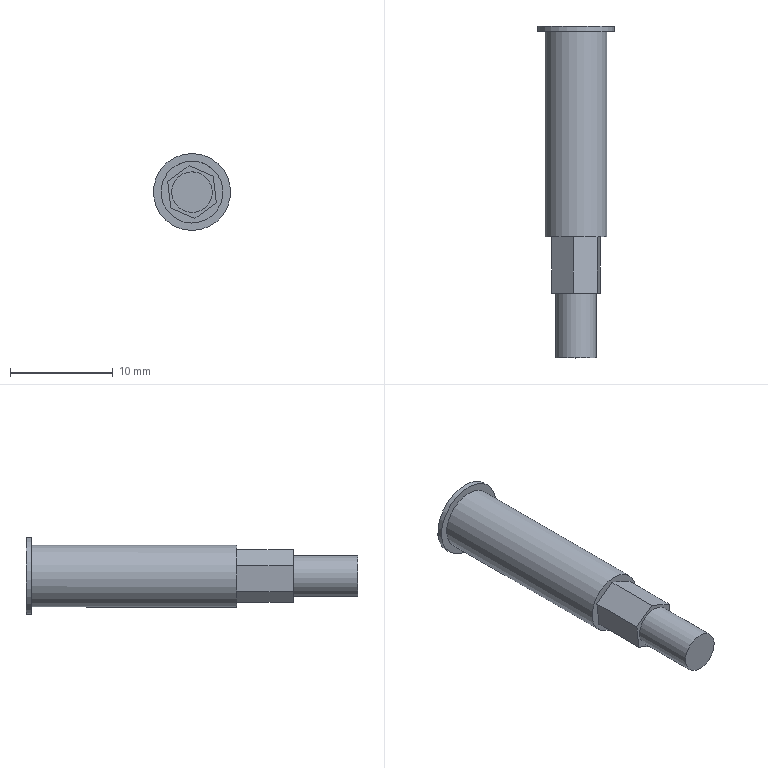Part | STEP file | Dodanie-wyci_gni_cie4_2 | 1 solid | 14 faces | box 7.5 x 32.302 x 7.5 mm | volume 765.405 mm3 | plane 11 | cylinder 3 | commonest cylinder face diameters 3.95 x1 6.03 x1 7.5 x1
STEP:
#1=CARTESIAN_POINT('',(0.,0.,0.));
#2=DIRECTION('',(0.,0.,1.));
#3=DIRECTION('',(1.,0.,0.));
#4=AXIS2_PLACEMENT_3D('',#1,#2,#3);
#5=CARTESIAN_POINT('',(158.273,-25.642,-123.21));
#6=VERTEX_POINT('',#5);
#7=CARTESIAN_POINT('',(158.273,-5.642,-123.202));
#8=VERTEX_POINT('',#7);
#9=CARTESIAN_POINT('',(158.273,-25.642,-123.21));
#10=DIRECTION('',(0.,1.,0.0003815));
#11=VECTOR('',#10,1.);
#12=LINE('',#9,#11);
#13=CARTESIAN_POINT('',(160.724,-5.642,-124.957));
#14=DIRECTION('',(0.,-1.,-0.0003815));
#15=DIRECTION('',(-0.8131,-0.0002221,0.5822));
#16=AXIS2_PLACEMENT_3D('',#13,#14,#15);
#17=CYLINDRICAL_SURFACE('',#16,3.015);
#18=CARTESIAN_POINT('',(0.000000001,20.));
#19=DIRECTION('',(0.,-1.));
#20=VECTOR('',#19,1.);
#21=LINE('',#18,#20);
#22=(GEOMETRIC_REPRESENTATION_CONTEXT(2)PARAMETRIC_REPRESENTATION_CONTEXT()REPRESENTATION_CONTEXT('',''));
#23=DEFINITIONAL_REPRESENTATION('',(#21),#22);
#24=PCURVE('',#17,#23);
#25=CARTESIAN_POINT('',(6.283,20.));
#26=DIRECTION('',(0.,-1.));
#27=VECTOR('',#26,1.);
#28=LINE('',#25,#27);
#29=(GEOMETRIC_REPRESENTATION_CONTEXT(2)PARAMETRIC_REPRESENTATION_CONTEXT()REPRESENTATION_CONTEXT('',''));
#30=DEFINITIONAL_REPRESENTATION('',(#28),#29);
#31=PCURVE('',#17,#30);
#32=SEAM_CURVE('',#12,(#24,#31),.PCURVE_S1.);
#33=EDGE_CURVE('',#6,#8,#32,.T.);
#34=ORIENTED_EDGE('',*,*,#33,.T.);
#35=CARTESIAN_POINT('',(160.724,-5.642,-124.957));
#36=DIRECTION('',(0.,-1.,-0.0003815));
#37=DIRECTION('',(-0.8131,-0.0002221,0.5822));
#38=AXIS2_PLACEMENT_3D('',#35,#36,#37);
#39=CIRCLE('',#38,3.015);
#40=CARTESIAN_POINT('',(0.,0.));
#41=DIRECTION('',(1.,0.));
#42=VECTOR('',#41,1.);
#43=LINE('',#40,#42);
#44=(GEOMETRIC_REPRESENTATION_CONTEXT(2)PARAMETRIC_REPRESENTATION_CONTEXT()REPRESENTATION_CONTEXT('',''));
#45=DEFINITIONAL_REPRESENTATION('',(#43),#44);
#46=PCURVE('',#17,#45);
#47=CARTESIAN_POINT('',(160.724,-5.642,-124.957));
#48=DIRECTION('',(0.,1.,0.0003815));
#49=DIRECTION('',(0.8131,0.0002221,-0.5822));
#50=AXIS2_PLACEMENT_3D('',#47,#48,#49);
#51=PLANE('',#50);
#52=CARTESIAN_POINT('',(-3.015,0.));
#53=CARTESIAN_POINT('',(-3.015,5.222));
#54=CARTESIAN_POINT('',(1.508,2.611));
#55=CARTESIAN_POINT('',(6.03,0.));
#56=CARTESIAN_POINT('',(1.508,-2.611));
#57=CARTESIAN_POINT('',(-3.015,-5.222));
#58=CARTESIAN_POINT('',(-3.015,0.));
#59=(BOUNDED_CURVE()B_SPLINE_CURVE(2,(#52,#53,#54,#55,#56,#57,#58),.UNSPECIFIED.,.T.,.F.)B_SPLINE_CURVE_WITH_KNOTS((1,2,2,2,2,1),(-2.094,0.,2.094,4.189,6.283,8.378),.UNSPECIFIED.)CURVE()GEOMETRIC_REPRESENTATION_ITEM()RATIONAL_B_SPLINE_CURVE((1.,0.5,1.,0.5,1.,0.5,1.))REPRESENTATION_ITEM(''));
#60=(GEOMETRIC_REPRESENTATION_CONTEXT(2)PARAMETRIC_REPRESENTATION_CONTEXT()REPRESENTATION_CONTEXT('',''));
#61=DEFINITIONAL_REPRESENTATION('',(#59),#60);
#62=PCURVE('',#51,#61);
#63=SURFACE_CURVE('',#39,(#46,#62),.PCURVE_S1.);
#64=EDGE_CURVE('',#8,#8,#63,.T.);
#65=ORIENTED_EDGE('',*,*,#64,.T.);
#66=ORIENTED_EDGE('',*,*,#33,.F.);
#67=CARTESIAN_POINT('',(160.724,-25.642,-124.965));
#68=DIRECTION('',(0.,1.,0.0003815));
#69=DIRECTION('',(-0.8131,-0.0002221,0.5822));
#70=AXIS2_PLACEMENT_3D('',#67,#68,#69);
#71=CIRCLE('',#70,3.015);
#72=CARTESIAN_POINT('',(6.283,20.));
#73=DIRECTION('',(-1.,0.));
#74=VECTOR('',#73,1.);
#75=LINE('',#72,#74);
#76=(GEOMETRIC_REPRESENTATION_CONTEXT(2)PARAMETRIC_REPRESENTATION_CONTEXT()REPRESENTATION_CONTEXT('',''));
#77=DEFINITIONAL_REPRESENTATION('',(#75),#76);
#78=PCURVE('',#17,#77);
#79=CARTESIAN_POINT('',(160.724,-25.642,-124.965));
#80=DIRECTION('',(0.,1.,0.0003815));
#81=DIRECTION('',(0.8131,0.0002221,-0.5822));
#82=AXIS2_PLACEMENT_3D('',#79,#80,#81);
#83=PLANE('',#82);
#84=CARTESIAN_POINT('',(0.,0.));
#85=DIRECTION('',(-1.,0.));
#86=AXIS2_PLACEMENT_2D('',#84,#85);
#87=CIRCLE('',#86,3.015);
#88=(GEOMETRIC_REPRESENTATION_CONTEXT(2)PARAMETRIC_REPRESENTATION_CONTEXT()REPRESENTATION_CONTEXT('',''));
#89=DEFINITIONAL_REPRESENTATION('',(#87),#88);
#90=PCURVE('',#83,#89);
#91=SURFACE_CURVE('',#71,(#78,#90),.PCURVE_S1.);
#92=EDGE_CURVE('',#6,#6,#91,.T.);
#93=ORIENTED_EDGE('',*,*,#92,.T.);
#94=EDGE_LOOP('',(#34,#65,#66,#93));
#95=FACE_BOUND('',#94,.T.);
#96=ADVANCED_FACE('',(#95),#17,.T.);
#97=CARTESIAN_POINT('',(157.675,-5.643,-122.774));
#98=VERTEX_POINT('',#97);
#99=CARTESIAN_POINT('',(157.675,-5.143,-122.774));
#100=VERTEX_POINT('',#99);
#101=CARTESIAN_POINT('',(157.675,-5.643,-122.774));
#102=DIRECTION('',(0.,1.,0.0003815));
#103=VECTOR('',#102,1.);
#104=LINE('',#101,#103);
#105=CARTESIAN_POINT('',(160.724,-5.142,-124.957));
#106=DIRECTION('',(0.,-1.,-0.0003815));
#107=DIRECTION('',(-0.8131,-0.0002221,0.5822));
#108=AXIS2_PLACEMENT_3D('',#105,#106,#107);
#109=CYLINDRICAL_SURFACE('',#108,3.75);
#110=CARTESIAN_POINT('',(0.,0.5));
#111=DIRECTION('',(0.,-1.));
#112=VECTOR('',#111,1.);
#113=LINE('',#110,#112);
#114=(GEOMETRIC_REPRESENTATION_CONTEXT(2)PARAMETRIC_REPRESENTATION_CONTEXT()REPRESENTATION_CONTEXT('',''));
#115=DEFINITIONAL_REPRESENTATION('',(#113),#114);
#116=PCURVE('',#109,#115);
#117=CARTESIAN_POINT('',(6.283,0.5));
#118=DIRECTION('',(0.,-1.));
#119=VECTOR('',#118,1.);
#120=LINE('',#117,#119);
#121=(GEOMETRIC_REPRESENTATION_CONTEXT(2)PARAMETRIC_REPRESENTATION_CONTEXT()REPRESENTATION_CONTEXT('',''));
#122=DEFINITIONAL_REPRESENTATION('',(#120),#121);
#123=PCURVE('',#109,#122);
#124=SEAM_CURVE('',#104,(#116,#123),.PCURVE_S1.);
#125=EDGE_CURVE('',#98,#100,#124,.T.);
#126=ORIENTED_EDGE('',*,*,#125,.T.);
#127=CARTESIAN_POINT('',(160.724,-5.142,-124.957));
#128=DIRECTION('',(0.,-1.,-0.0003815));
#129=DIRECTION('',(-0.8131,-0.0002221,0.5822));
#130=AXIS2_PLACEMENT_3D('',#127,#128,#129);
#131=CIRCLE('',#130,3.75);
#132=CARTESIAN_POINT('',(0.,0.));
#133=DIRECTION('',(1.,0.));
#134=VECTOR('',#133,1.);
#135=LINE('',#132,#134);
#136=(GEOMETRIC_REPRESENTATION_CONTEXT(2)PARAMETRIC_REPRESENTATION_CONTEXT()REPRESENTATION_CONTEXT('',''));
#137=DEFINITIONAL_REPRESENTATION('',(#135),#136);
#138=PCURVE('',#109,#137);
#139=CARTESIAN_POINT('',(160.724,-5.142,-124.957));
#140=DIRECTION('',(0.,1.,0.0003815));
#141=DIRECTION('',(0.8131,0.0002221,-0.5822));
#142=AXIS2_PLACEMENT_3D('',#139,#140,#141);
#143=PLANE('',#142);
#144=CARTESIAN_POINT('',(-3.75,0.));
#145=CARTESIAN_POINT('',(-3.75,6.495));
#146=CARTESIAN_POINT('',(1.875,3.248));
#147=CARTESIAN_POINT('',(7.5,0.));
#148=CARTESIAN_POINT('',(1.875,-3.248));
#149=CARTESIAN_POINT('',(-3.75,-6.495));
#150=CARTESIAN_POINT('',(-3.75,0.));
#151=(BOUNDED_CURVE()B_SPLINE_CURVE(2,(#144,#145,#146,#147,#148,#149,#150),.UNSPECIFIED.,.T.,.F.)B_SPLINE_CURVE_WITH_KNOTS((1,2,2,2,2,1),(-2.094,0.,2.094,4.189,6.283,8.378),.UNSPECIFIED.)CURVE()GEOMETRIC_REPRESENTATION_ITEM()RATIONAL_B_SPLINE_CURVE((1.,0.5,1.,0.5,1.,0.5,1.))REPRESENTATION_ITEM(''));
#152=(GEOMETRIC_REPRESENTATION_CONTEXT(2)PARAMETRIC_REPRESENTATION_CONTEXT()REPRESENTATION_CONTEXT('',''));
#153=DEFINITIONAL_REPRESENTATION('',(#151),#152);
#154=PCURVE('',#143,#153);
#155=SURFACE_CURVE('',#131,(#138,#154),.PCURVE_S1.);
#156=EDGE_CURVE('',#100,#100,#155,.T.);
#157=ORIENTED_EDGE('',*,*,#156,.T.);
#158=ORIENTED_EDGE('',*,*,#125,.F.);
#159=CARTESIAN_POINT('',(160.724,-5.642,-124.957));
#160=DIRECTION('',(0.,1.,0.0003815));
#161=DIRECTION('',(-0.8131,-0.0002221,0.5822));
#162=AXIS2_PLACEMENT_3D('',#159,#160,#161);
#163=CIRCLE('',#162,3.75);
#164=CARTESIAN_POINT('',(6.283,0.5));
#165=DIRECTION('',(-1.,0.));
#166=VECTOR('',#165,1.);
#167=LINE('',#164,#166);
#168=(GEOMETRIC_REPRESENTATION_CONTEXT(2)PARAMETRIC_REPRESENTATION_CONTEXT()REPRESENTATION_CONTEXT('',''));
#169=DEFINITIONAL_REPRESENTATION('',(#167),#168);
#170=PCURVE('',#109,#169);
#171=CARTESIAN_POINT('',(0.,0.));
#172=DIRECTION('',(-1.,0.));
#173=AXIS2_PLACEMENT_2D('',#171,#172);
#174=CIRCLE('',#173,3.75);
#175=(GEOMETRIC_REPRESENTATION_CONTEXT(2)PARAMETRIC_REPRESENTATION_CONTEXT()REPRESENTATION_CONTEXT('',''));
#176=DEFINITIONAL_REPRESENTATION('',(#174),#175);
#177=PCURVE('',#51,#176);
#178=SURFACE_CURVE('',#163,(#170,#177),.PCURVE_S1.);
#179=EDGE_CURVE('',#98,#98,#178,.T.);
#180=ORIENTED_EDGE('',*,*,#179,.T.);
#181=EDGE_LOOP('',(#126,#157,#158,#180));
#182=FACE_BOUND('',#181,.T.);
#183=ADVANCED_FACE('',(#182),#109,.T.);
#184=CARTESIAN_POINT('',(159.118,-37.442,-123.82));
#185=VERTEX_POINT('',#184);
#186=CARTESIAN_POINT('',(159.118,-31.142,-123.817));
#187=VERTEX_POINT('',#186);
#188=CARTESIAN_POINT('',(159.118,-37.442,-123.82));
#189=DIRECTION('',(0.,1.,0.0003815));
#190=VECTOR('',#189,1.);
#191=LINE('',#188,#190);
#192=CARTESIAN_POINT('',(160.724,-31.142,-124.967));
#193=DIRECTION('',(0.,-1.,-0.0003815));
#194=DIRECTION('',(-0.8131,-0.0002221,0.5822));
#195=AXIS2_PLACEMENT_3D('',#192,#193,#194);
#196=CYLINDRICAL_SURFACE('',#195,1.975);
#197=CARTESIAN_POINT('',(0.,6.3));
#198=DIRECTION('',(0.,-1.));
#199=VECTOR('',#198,1.);
#200=LINE('',#197,#199);
#201=(GEOMETRIC_REPRESENTATION_CONTEXT(2)PARAMETRIC_REPRESENTATION_CONTEXT()REPRESENTATION_CONTEXT('',''));
#202=DEFINITIONAL_REPRESENTATION('',(#200),#201);
#203=PCURVE('',#196,#202);
#204=CARTESIAN_POINT('',(6.283,6.3));
#205=DIRECTION('',(0.,-1.));
#206=VECTOR('',#205,1.);
#207=LINE('',#204,#206);
#208=(GEOMETRIC_REPRESENTATION_CONTEXT(2)PARAMETRIC_REPRESENTATION_CONTEXT()REPRESENTATION_CONTEXT('',''));
#209=DEFINITIONAL_REPRESENTATION('',(#207),#208);
#210=PCURVE('',#196,#209);
#211=SEAM_CURVE('',#191,(#203,#210),.PCURVE_S1.);
#212=EDGE_CURVE('',#185,#187,#211,.T.);
#213=ORIENTED_EDGE('',*,*,#212,.T.);
#214=CARTESIAN_POINT('',(160.724,-31.142,-124.967));
#215=DIRECTION('',(0.,-1.,-0.0003815));
#216=DIRECTION('',(-0.8131,-0.0002221,0.5822));
#217=AXIS2_PLACEMENT_3D('',#214,#215,#216);
#218=CIRCLE('',#217,1.975);
#219=CARTESIAN_POINT('',(0.,0.));
#220=DIRECTION('',(1.,0.));
#221=VECTOR('',#220,1.);
#222=LINE('',#219,#221);
#223=(GEOMETRIC_REPRESENTATION_CONTEXT(2)PARAMETRIC_REPRESENTATION_CONTEXT()REPRESENTATION_CONTEXT('',''));
#224=DEFINITIONAL_REPRESENTATION('',(#222),#223);
#225=PCURVE('',#196,#224);
#226=CARTESIAN_POINT('',(160.724,-31.142,-124.967));
#227=DIRECTION('',(0.,1.,0.0003815));
#228=DIRECTION('',(0.8131,0.0002221,-0.5822));
#229=AXIS2_PLACEMENT_3D('',#226,#227,#228);
#230=PLANE('',#229);
#231=CARTESIAN_POINT('',(-1.975,0.));
#232=CARTESIAN_POINT('',(-1.975,3.421));
#233=CARTESIAN_POINT('',(0.9875,1.71));
#234=CARTESIAN_POINT('',(3.95,0.));
#235=CARTESIAN_POINT('',(0.9875,-1.71));
#236=CARTESIAN_POINT('',(-1.975,-3.421));
#237=CARTESIAN_POINT('',(-1.975,0.));
#238=(BOUNDED_CURVE()B_SPLINE_CURVE(2,(#231,#232,#233,#234,#235,#236,#237),.UNSPECIFIED.,.T.,.F.)B_SPLINE_CURVE_WITH_KNOTS((1,2,2,2,2,1),(-2.094,0.,2.094,4.189,6.283,8.378),.UNSPECIFIED.)CURVE()GEOMETRIC_REPRESENTATION_ITEM()RATIONAL_B_SPLINE_CURVE((1.,0.5,1.,0.5,1.,0.5,1.))REPRESENTATION_ITEM(''));
#239=(GEOMETRIC_REPRESENTATION_CONTEXT(2)PARAMETRIC_REPRESENTATION_CONTEXT()REPRESENTATION_CONTEXT('',''));
#240=DEFINITIONAL_REPRESENTATION('',(#238),#239);
#241=PCURVE('',#230,#240);
#242=SURFACE_CURVE('',#218,(#225,#241),.PCURVE_S1.);
#243=EDGE_CURVE('',#187,#187,#242,.T.);
#244=ORIENTED_EDGE('',*,*,#243,.T.);
#245=ORIENTED_EDGE('',*,*,#212,.F.);
#246=CARTESIAN_POINT('',(160.724,-37.442,-124.969));
#247=DIRECTION('',(0.,1.,0.0003815));
#248=DIRECTION('',(-0.8131,-0.0002221,0.5822));
#249=AXIS2_PLACEMENT_3D('',#246,#247,#248);
#250=CIRCLE('',#249,1.975);
#251=CARTESIAN_POINT('',(6.283,6.3));
#252=DIRECTION('',(-1.,0.));
#253=VECTOR('',#252,1.);
#254=LINE('',#251,#253);
#255=(GEOMETRIC_REPRESENTATION_CONTEXT(2)PARAMETRIC_REPRESENTATION_CONTEXT()REPRESENTATION_CONTEXT('',''));
#256=DEFINITIONAL_REPRESENTATION('',(#254),#255);
#257=PCURVE('',#196,#256);
#258=CARTESIAN_POINT('',(160.724,-37.442,-124.969));
#259=DIRECTION('',(0.,1.,0.0003815));
#260=DIRECTION('',(0.8131,0.0002221,-0.5822));
#261=AXIS2_PLACEMENT_3D('',#258,#259,#260);
#262=PLANE('',#261);
#263=CARTESIAN_POINT('',(0.,0.));
#264=DIRECTION('',(-1.,0.));
#265=AXIS2_PLACEMENT_2D('',#263,#264);
#266=CIRCLE('',#265,1.975);
#267=(GEOMETRIC_REPRESENTATION_CONTEXT(2)PARAMETRIC_REPRESENTATION_CONTEXT()REPRESENTATION_CONTEXT('',''));
#268=DEFINITIONAL_REPRESENTATION('',(#266),#267);
#269=PCURVE('',#262,#268);
#270=SURFACE_CURVE('',#250,(#257,#269),.PCURVE_S1.);
#271=EDGE_CURVE('',#185,#185,#270,.T.);
#272=ORIENTED_EDGE('',*,*,#271,.T.);
#273=EDGE_LOOP('',(#213,#244,#245,#272));
#274=FACE_BOUND('',#273,.T.);
#275=ADVANCED_FACE('',(#274),#196,.T.);
#276=CARTESIAN_POINT('',(161.015,-25.641,-127.526));
#277=VERTEX_POINT('',#276);
#278=CARTESIAN_POINT('',(163.088,-25.641,-125.994));
#279=VERTEX_POINT('',#278);
#280=CARTESIAN_POINT('',(161.015,-25.641,-127.526));
#281=DIRECTION('',(0.8042,-0.0002268,0.5944));
#282=VECTOR('',#281,1.);
#283=LINE('',#280,#282);
#284=CARTESIAN_POINT('',(1.727,1.913));
#285=DIRECTION('',(0.3078,-0.9515));
#286=VECTOR('',#285,1.);
#287=LINE('',#284,#286);
#288=(GEOMETRIC_REPRESENTATION_CONTEXT(2)PARAMETRIC_REPRESENTATION_CONTEXT()REPRESENTATION_CONTEXT('',''));
#289=DEFINITIONAL_REPRESENTATION('',(#287),#288);
#290=PCURVE('',#83,#289);
#291=CARTESIAN_POINT('',(162.051,-28.391,-126.761));
#292=DIRECTION('',(-0.5944,-0.0003068,0.8042));
#293=DIRECTION('',(0.8042,-0.0002268,0.5944));
#294=AXIS2_PLACEMENT_3D('',#291,#292,#293);
#295=PLANE('',#294);
#296=CARTESIAN_POINT('',(-1.289,2.75));
#297=DIRECTION('',(1.,0.));
#298=VECTOR('',#297,1.);
#299=LINE('',#296,#298);
#300=(GEOMETRIC_REPRESENTATION_CONTEXT(2)PARAMETRIC_REPRESENTATION_CONTEXT()REPRESENTATION_CONTEXT('',''));
#301=DEFINITIONAL_REPRESENTATION('',(#299),#300);
#302=PCURVE('',#295,#301);
#303=SURFACE_CURVE('',#283,(#290,#302),.PCURVE_S1.);
#304=EDGE_CURVE('',#277,#279,#303,.T.);
#305=ORIENTED_EDGE('',*,*,#304,.F.);
#306=CARTESIAN_POINT('',(158.651,-25.641,-126.497));
#307=VERTEX_POINT('',#306);
#308=CARTESIAN_POINT('',(158.651,-25.641,-126.497));
#309=DIRECTION('',(0.9169,0.0001523,-0.3992));
#310=VECTOR('',#309,1.);
#311=LINE('',#308,#310);
#312=CARTESIAN_POINT('',(-0.7934,2.453));
#313=DIRECTION('',(0.9779,-0.2092));
#314=VECTOR('',#313,1.);
#315=LINE('',#312,#314);
#316=(GEOMETRIC_REPRESENTATION_CONTEXT(2)PARAMETRIC_REPRESENTATION_CONTEXT()REPRESENTATION_CONTEXT('',''));
#317=DEFINITIONAL_REPRESENTATION('',(#315),#316);
#318=PCURVE('',#83,#317);
#319=CARTESIAN_POINT('',(159.833,-28.391,-127.013));
#320=DIRECTION('',(0.3992,-0.0003498,0.9169));
#321=DIRECTION('',(0.9169,0.0001523,-0.3992));
#322=AXIS2_PLACEMENT_3D('',#319,#320,#321);
#323=PLANE('',#322);
#324=CARTESIAN_POINT('',(-1.289,2.75));
#325=DIRECTION('',(1.,0.));
#326=VECTOR('',#325,1.);
#327=LINE('',#324,#326);
#328=(GEOMETRIC_REPRESENTATION_CONTEXT(2)PARAMETRIC_REPRESENTATION_CONTEXT()REPRESENTATION_CONTEXT('',''));
#329=DEFINITIONAL_REPRESENTATION('',(#327),#328);
#330=PCURVE('',#323,#329);
#331=SURFACE_CURVE('',#311,(#318,#330),.PCURVE_S1.);
#332=EDGE_CURVE('',#307,#277,#331,.T.);
#333=ORIENTED_EDGE('',*,*,#332,.F.);
#334=CARTESIAN_POINT('',(158.361,-25.642,-123.936));
#335=VERTEX_POINT('',#334);
#336=CARTESIAN_POINT('',(158.361,-25.642,-123.936));
#337=DIRECTION('',(0.1127,0.000379,-0.9936));
#338=VECTOR('',#337,1.);
#339=LINE('',#336,#338);
#340=CARTESIAN_POINT('',(-2.521,0.5392));
#341=DIRECTION('',(0.6701,0.7423));
#342=VECTOR('',#341,1.);
#343=LINE('',#340,#342);
#344=(GEOMETRIC_REPRESENTATION_CONTEXT(2)PARAMETRIC_REPRESENTATION_CONTEXT()REPRESENTATION_CONTEXT('',''));
#345=DEFINITIONAL_REPRESENTATION('',(#343),#344);
#346=PCURVE('',#83,#345);
#347=CARTESIAN_POINT('',(158.506,-28.392,-125.218));
#348=DIRECTION('',(0.9936,-0.00004299,0.1127));
#349=DIRECTION('',(0.1127,0.000379,-0.9936));
#350=AXIS2_PLACEMENT_3D('',#347,#348,#349);
#351=PLANE('',#350);
#352=CARTESIAN_POINT('',(-1.289,2.75));
#353=DIRECTION('',(1.,0.));
#354=VECTOR('',#353,1.);
#355=LINE('',#352,#354);
#356=(GEOMETRIC_REPRESENTATION_CONTEXT(2)PARAMETRIC_REPRESENTATION_CONTEXT()REPRESENTATION_CONTEXT('',''));
#357=DEFINITIONAL_REPRESENTATION('',(#355),#356);
#358=PCURVE('',#351,#357);
#359=SURFACE_CURVE('',#339,(#346,#358),.PCURVE_S1.);
#360=EDGE_CURVE('',#335,#307,#359,.T.);
#361=ORIENTED_EDGE('',*,*,#360,.F.);
#362=CARTESIAN_POINT('',(160.434,-25.643,-122.404));
#363=VERTEX_POINT('',#362);
#364=CARTESIAN_POINT('',(160.434,-25.643,-122.404));
#365=DIRECTION('',(-0.8042,0.0002268,-0.5944));
#366=VECTOR('',#365,1.);
#367=LINE('',#364,#366);
#368=CARTESIAN_POINT('',(-1.727,-1.913));
#369=DIRECTION('',(-0.3078,0.9515));
#370=VECTOR('',#369,1.);
#371=LINE('',#368,#370);
#372=(GEOMETRIC_REPRESENTATION_CONTEXT(2)PARAMETRIC_REPRESENTATION_CONTEXT()REPRESENTATION_CONTEXT('',''));
#373=DEFINITIONAL_REPRESENTATION('',(#371),#372);
#374=PCURVE('',#83,#373);
#375=CARTESIAN_POINT('',(159.397,-28.392,-123.171));
#376=DIRECTION('',(0.5944,0.0003068,-0.8042));
#377=DIRECTION('',(-0.8042,0.0002268,-0.5944));
#378=AXIS2_PLACEMENT_3D('',#375,#376,#377);
#379=PLANE('',#378);
#380=CARTESIAN_POINT('',(-1.289,2.75));
#381=DIRECTION('',(1.,0.));
#382=VECTOR('',#381,1.);
#383=LINE('',#380,#382);
#384=(GEOMETRIC_REPRESENTATION_CONTEXT(2)PARAMETRIC_REPRESENTATION_CONTEXT()REPRESENTATION_CONTEXT('',''));
#385=DEFINITIONAL_REPRESENTATION('',(#383),#384);
#386=PCURVE('',#379,#385);
#387=SURFACE_CURVE('',#367,(#374,#386),.PCURVE_S1.);
#388=EDGE_CURVE('',#363,#335,#387,.T.);
#389=ORIENTED_EDGE('',*,*,#388,.F.);
#390=CARTESIAN_POINT('',(162.797,-25.642,-123.433));
#391=VERTEX_POINT('',#390);
#392=CARTESIAN_POINT('',(162.797,-25.642,-123.433));
#393=DIRECTION('',(-0.9169,-0.0001523,0.3992));
#394=VECTOR('',#393,1.);
#395=LINE('',#392,#394);
#396=CARTESIAN_POINT('',(0.7934,-2.453));
#397=DIRECTION('',(-0.9779,0.2092));
#398=VECTOR('',#397,1.);
#399=LINE('',#396,#398);
#400=(GEOMETRIC_REPRESENTATION_CONTEXT(2)PARAMETRIC_REPRESENTATION_CONTEXT()REPRESENTATION_CONTEXT('',''));
#401=DEFINITIONAL_REPRESENTATION('',(#399),#400);
#402=PCURVE('',#83,#401);
#403=CARTESIAN_POINT('',(161.615,-28.393,-122.919));
#404=DIRECTION('',(-0.3992,0.0003498,-0.9169));
#405=DIRECTION('',(-0.9169,-0.0001523,0.3992));
#406=AXIS2_PLACEMENT_3D('',#403,#404,#405);
#407=PLANE('',#406);
#408=CARTESIAN_POINT('',(-1.289,2.75));
#409=DIRECTION('',(1.,0.));
#410=VECTOR('',#409,1.);
#411=LINE('',#408,#410);
#412=(GEOMETRIC_REPRESENTATION_CONTEXT(2)PARAMETRIC_REPRESENTATION_CONTEXT()REPRESENTATION_CONTEXT('',''));
#413=DEFINITIONAL_REPRESENTATION('',(#411),#412);
#414=PCURVE('',#407,#413);
#415=SURFACE_CURVE('',#395,(#402,#414),.PCURVE_S1.);
#416=EDGE_CURVE('',#391,#363,#415,.T.);
#417=ORIENTED_EDGE('',*,*,#416,.F.);
#418=CARTESIAN_POINT('',(163.088,-25.641,-125.994));
#419=DIRECTION('',(-0.1127,-0.000379,0.9936));
#420=VECTOR('',#419,1.);
#421=LINE('',#418,#420);
#422=CARTESIAN_POINT('',(2.521,-0.5392));
#423=DIRECTION('',(-0.6701,-0.7423));
#424=VECTOR('',#423,1.);
#425=LINE('',#422,#424);
#426=(GEOMETRIC_REPRESENTATION_CONTEXT(2)PARAMETRIC_REPRESENTATION_CONTEXT()REPRESENTATION_CONTEXT('',''));
#427=DEFINITIONAL_REPRESENTATION('',(#425),#426);
#428=PCURVE('',#83,#427);
#429=CARTESIAN_POINT('',(162.942,-28.392,-124.714));
#430=DIRECTION('',(-0.9936,0.00004299,-0.1127));
#431=DIRECTION('',(-0.1127,-0.000379,0.9936));
#432=AXIS2_PLACEMENT_3D('',#429,#430,#431);
#433=PLANE('',#432);
#434=CARTESIAN_POINT('',(-1.289,2.75));
#435=DIRECTION('',(1.,0.));
#436=VECTOR('',#435,1.);
#437=LINE('',#434,#436);
#438=(GEOMETRIC_REPRESENTATION_CONTEXT(2)PARAMETRIC_REPRESENTATION_CONTEXT()REPRESENTATION_CONTEXT('',''));
#439=DEFINITIONAL_REPRESENTATION('',(#437),#438);
#440=PCURVE('',#433,#439);
#441=SURFACE_CURVE('',#421,(#428,#440),.PCURVE_S1.);
#442=EDGE_CURVE('',#279,#391,#441,.T.);
#443=ORIENTED_EDGE('',*,*,#442,.F.);
#444=EDGE_LOOP('',(#305,#333,#361,#389,#417,#443));
#445=FACE_BOUND('',#444,.T.);
#446=ORIENTED_EDGE('',*,*,#92,.F.);
#447=EDGE_LOOP('',(#446));
#448=FACE_BOUND('',#447,.T.);
#449=ADVANCED_FACE('',(#445,#448),#83,.F.);
#450=ORIENTED_EDGE('',*,*,#64,.F.);
#451=EDGE_LOOP('',(#450));
#452=FACE_BOUND('',#451,.T.);
#453=ORIENTED_EDGE('',*,*,#179,.F.);
#454=EDGE_LOOP('',(#453));
#455=FACE_BOUND('',#454,.T.);
#456=ADVANCED_FACE('',(#452,#455),#51,.F.);
#457=CARTESIAN_POINT('',(163.088,-31.141,-125.996));
#458=VERTEX_POINT('',#457);
#459=CARTESIAN_POINT('',(163.088,-25.641,-125.994));
#460=DIRECTION('',(0.,-1.,-0.0003815));
#461=VECTOR('',#460,1.);
#462=LINE('',#459,#461);
#463=CARTESIAN_POINT('',(-1.289,2.75));
#464=DIRECTION('',(0.,-1.));
#465=VECTOR('',#464,1.);
#466=LINE('',#463,#465);
#467=(GEOMETRIC_REPRESENTATION_CONTEXT(2)PARAMETRIC_REPRESENTATION_CONTEXT()REPRESENTATION_CONTEXT('',''));
#468=DEFINITIONAL_REPRESENTATION('',(#466),#467);
#469=PCURVE('',#433,#468);
#470=CARTESIAN_POINT('',(1.289,2.75));
#471=DIRECTION('',(0.,-1.));
#472=VECTOR('',#471,1.);
#473=LINE('',#470,#472);
#474=(GEOMETRIC_REPRESENTATION_CONTEXT(2)PARAMETRIC_REPRESENTATION_CONTEXT()REPRESENTATION_CONTEXT('',''));
#475=DEFINITIONAL_REPRESENTATION('',(#473),#474);
#476=PCURVE('',#295,#475);
#477=SURFACE_CURVE('',#462,(#469,#476),.PCURVE_S1.);
#478=EDGE_CURVE('',#279,#458,#477,.T.);
#479=ORIENTED_EDGE('',*,*,#478,.F.);
#480=ORIENTED_EDGE('',*,*,#442,.T.);
#481=CARTESIAN_POINT('',(162.797,-31.142,-123.435));
#482=VERTEX_POINT('',#481);
#483=CARTESIAN_POINT('',(162.797,-31.142,-123.435));
#484=DIRECTION('',(0.,1.,0.0003815));
#485=VECTOR('',#484,1.);
#486=LINE('',#483,#485);
#487=CARTESIAN_POINT('',(1.289,-2.75));
#488=DIRECTION('',(0.,1.));
#489=VECTOR('',#488,1.);
#490=LINE('',#487,#489);
#491=(GEOMETRIC_REPRESENTATION_CONTEXT(2)PARAMETRIC_REPRESENTATION_CONTEXT()REPRESENTATION_CONTEXT('',''));
#492=DEFINITIONAL_REPRESENTATION('',(#490),#491);
#493=PCURVE('',#433,#492);
#494=CARTESIAN_POINT('',(-1.289,-2.75));
#495=DIRECTION('',(0.,1.));
#496=VECTOR('',#495,1.);
#497=LINE('',#494,#496);
#498=(GEOMETRIC_REPRESENTATION_CONTEXT(2)PARAMETRIC_REPRESENTATION_CONTEXT()REPRESENTATION_CONTEXT('',''));
#499=DEFINITIONAL_REPRESENTATION('',(#497),#498);
#500=PCURVE('',#407,#499);
#501=SURFACE_CURVE('',#486,(#493,#500),.PCURVE_S1.);
#502=EDGE_CURVE('',#482,#391,#501,.T.);
#503=ORIENTED_EDGE('',*,*,#502,.F.);
#504=CARTESIAN_POINT('',(163.088,-31.141,-125.996));
#505=DIRECTION('',(-0.1127,-0.000379,0.9936));
#506=VECTOR('',#505,1.);
#507=LINE('',#504,#506);
#508=CARTESIAN_POINT('',(-1.289,-2.75));
#509=DIRECTION('',(1.,0.));
#510=VECTOR('',#509,1.);
#511=LINE('',#508,#510);
#512=(GEOMETRIC_REPRESENTATION_CONTEXT(2)PARAMETRIC_REPRESENTATION_CONTEXT()REPRESENTATION_CONTEXT('',''));
#513=DEFINITIONAL_REPRESENTATION('',(#511),#512);
#514=PCURVE('',#433,#513);
#515=CARTESIAN_POINT('',(2.521,-0.5392));
#516=DIRECTION('',(-0.6701,-0.7423));
#517=VECTOR('',#516,1.);
#518=LINE('',#515,#517);
#519=(GEOMETRIC_REPRESENTATION_CONTEXT(2)PARAMETRIC_REPRESENTATION_CONTEXT()REPRESENTATION_CONTEXT('',''));
#520=DEFINITIONAL_REPRESENTATION('',(#518),#519);
#521=PCURVE('',#230,#520);
#522=SURFACE_CURVE('',#507,(#514,#521),.PCURVE_S1.);
#523=EDGE_CURVE('',#458,#482,#522,.T.);
#524=ORIENTED_EDGE('',*,*,#523,.F.);
#525=EDGE_LOOP('',(#479,#480,#503,#524));
#526=FACE_BOUND('',#525,.T.);
#527=ADVANCED_FACE('',(#526),#433,.F.);
#528=CARTESIAN_POINT('',(161.015,-31.141,-127.529));
#529=VERTEX_POINT('',#528);
#530=CARTESIAN_POINT('',(161.015,-25.641,-127.526));
#531=DIRECTION('',(0.,-1.,-0.0003815));
#532=VECTOR('',#531,1.);
#533=LINE('',#530,#532);
#534=CARTESIAN_POINT('',(-1.289,2.75));
#535=DIRECTION('',(0.,-1.));
#536=VECTOR('',#535,1.);
#537=LINE('',#534,#536);
#538=(GEOMETRIC_REPRESENTATION_CONTEXT(2)PARAMETRIC_REPRESENTATION_CONTEXT()REPRESENTATION_CONTEXT('',''));
#539=DEFINITIONAL_REPRESENTATION('',(#537),#538);
#540=PCURVE('',#295,#539);
#541=CARTESIAN_POINT('',(1.289,2.75));
#542=DIRECTION('',(0.,-1.));
#543=VECTOR('',#542,1.);
#544=LINE('',#541,#543);
#545=(GEOMETRIC_REPRESENTATION_CONTEXT(2)PARAMETRIC_REPRESENTATION_CONTEXT()REPRESENTATION_CONTEXT('',''));
#546=DEFINITIONAL_REPRESENTATION('',(#544),#545);
#547=PCURVE('',#323,#546);
#548=SURFACE_CURVE('',#533,(#540,#547),.PCURVE_S1.);
#549=EDGE_CURVE('',#277,#529,#548,.T.);
#550=ORIENTED_EDGE('',*,*,#549,.F.);
#551=ORIENTED_EDGE('',*,*,#304,.T.);
#552=ORIENTED_EDGE('',*,*,#478,.T.);
#553=CARTESIAN_POINT('',(161.015,-31.141,-127.529));
#554=DIRECTION('',(0.8042,-0.0002268,0.5944));
#555=VECTOR('',#554,1.);
#556=LINE('',#553,#555);
#557=CARTESIAN_POINT('',(-1.289,-2.75));
#558=DIRECTION('',(1.,0.));
#559=VECTOR('',#558,1.);
#560=LINE('',#557,#559);
#561=(GEOMETRIC_REPRESENTATION_CONTEXT(2)PARAMETRIC_REPRESENTATION_CONTEXT()REPRESENTATION_CONTEXT('',''));
#562=DEFINITIONAL_REPRESENTATION('',(#560),#561);
#563=PCURVE('',#295,#562);
#564=CARTESIAN_POINT('',(1.727,1.913));
#565=DIRECTION('',(0.3078,-0.9515));
#566=VECTOR('',#565,1.);
#567=LINE('',#564,#566);
#568=(GEOMETRIC_REPRESENTATION_CONTEXT(2)PARAMETRIC_REPRESENTATION_CONTEXT()REPRESENTATION_CONTEXT('',''));
#569=DEFINITIONAL_REPRESENTATION('',(#567),#568);
#570=PCURVE('',#230,#569);
#571=SURFACE_CURVE('',#556,(#563,#570),.PCURVE_S1.);
#572=EDGE_CURVE('',#529,#458,#571,.T.);
#573=ORIENTED_EDGE('',*,*,#572,.F.);
#574=EDGE_LOOP('',(#550,#551,#552,#573));
#575=FACE_BOUND('',#574,.T.);
#576=ADVANCED_FACE('',(#575),#295,.F.);
#577=CARTESIAN_POINT('',(158.651,-31.141,-126.499));
#578=VERTEX_POINT('',#577);
#579=CARTESIAN_POINT('',(158.651,-25.641,-126.497));
#580=DIRECTION('',(0.,-1.,-0.0003815));
#581=VECTOR('',#580,1.);
#582=LINE('',#579,#581);
#583=CARTESIAN_POINT('',(-1.289,2.75));
#584=DIRECTION('',(0.,-1.));
#585=VECTOR('',#584,1.);
#586=LINE('',#583,#585);
#587=(GEOMETRIC_REPRESENTATION_CONTEXT(2)PARAMETRIC_REPRESENTATION_CONTEXT()REPRESENTATION_CONTEXT('',''));
#588=DEFINITIONAL_REPRESENTATION('',(#586),#587);
#589=PCURVE('',#323,#588);
#590=CARTESIAN_POINT('',(1.289,2.75));
#591=DIRECTION('',(0.,-1.));
#592=VECTOR('',#591,1.);
#593=LINE('',#590,#592);
#594=(GEOMETRIC_REPRESENTATION_CONTEXT(2)PARAMETRIC_REPRESENTATION_CONTEXT()REPRESENTATION_CONTEXT('',''));
#595=DEFINITIONAL_REPRESENTATION('',(#593),#594);
#596=PCURVE('',#351,#595);
#597=SURFACE_CURVE('',#582,(#589,#596),.PCURVE_S1.);
#598=EDGE_CURVE('',#307,#578,#597,.T.);
#599=ORIENTED_EDGE('',*,*,#598,.F.);
#600=ORIENTED_EDGE('',*,*,#332,.T.);
#601=ORIENTED_EDGE('',*,*,#549,.T.);
#602=CARTESIAN_POINT('',(158.651,-31.141,-126.499));
#603=DIRECTION('',(0.9169,0.0001523,-0.3992));
#604=VECTOR('',#603,1.);
#605=LINE('',#602,#604);
#606=CARTESIAN_POINT('',(-1.289,-2.75));
#607=DIRECTION('',(1.,0.));
#608=VECTOR('',#607,1.);
#609=LINE('',#606,#608);
#610=(GEOMETRIC_REPRESENTATION_CONTEXT(2)PARAMETRIC_REPRESENTATION_CONTEXT()REPRESENTATION_CONTEXT('',''));
#611=DEFINITIONAL_REPRESENTATION('',(#609),#610);
#612=PCURVE('',#323,#611);
#613=CARTESIAN_POINT('',(-0.7934,2.453));
#614=DIRECTION('',(0.9779,-0.2092));
#615=VECTOR('',#614,1.);
#616=LINE('',#613,#615);
#617=(GEOMETRIC_REPRESENTATION_CONTEXT(2)PARAMETRIC_REPRESENTATION_CONTEXT()REPRESENTATION_CONTEXT('',''));
#618=DEFINITIONAL_REPRESENTATION('',(#616),#617);
#619=PCURVE('',#230,#618);
#620=SURFACE_CURVE('',#605,(#612,#619),.PCURVE_S1.);
#621=EDGE_CURVE('',#578,#529,#620,.T.);
#622=ORIENTED_EDGE('',*,*,#621,.F.);
#623=EDGE_LOOP('',(#599,#600,#601,#622));
#624=FACE_BOUND('',#623,.T.);
#625=ADVANCED_FACE('',(#624),#323,.F.);
#626=CARTESIAN_POINT('',(158.361,-31.142,-123.938));
#627=VERTEX_POINT('',#626);
#628=CARTESIAN_POINT('',(158.361,-25.642,-123.936));
#629=DIRECTION('',(0.,-1.,-0.0003815));
#630=VECTOR('',#629,1.);
#631=LINE('',#628,#630);
#632=CARTESIAN_POINT('',(-1.289,2.75));
#633=DIRECTION('',(0.,-1.));
#634=VECTOR('',#633,1.);
#635=LINE('',#632,#634);
#636=(GEOMETRIC_REPRESENTATION_CONTEXT(2)PARAMETRIC_REPRESENTATION_CONTEXT()REPRESENTATION_CONTEXT('',''));
#637=DEFINITIONAL_REPRESENTATION('',(#635),#636);
#638=PCURVE('',#351,#637);
#639=CARTESIAN_POINT('',(1.289,2.75));
#640=DIRECTION('',(0.,-1.));
#641=VECTOR('',#640,1.);
#642=LINE('',#639,#641);
#643=(GEOMETRIC_REPRESENTATION_CONTEXT(2)PARAMETRIC_REPRESENTATION_CONTEXT()REPRESENTATION_CONTEXT('',''));
#644=DEFINITIONAL_REPRESENTATION('',(#642),#643);
#645=PCURVE('',#379,#644);
#646=SURFACE_CURVE('',#631,(#638,#645),.PCURVE_S1.);
#647=EDGE_CURVE('',#335,#627,#646,.T.);
#648=ORIENTED_EDGE('',*,*,#647,.F.);
#649=ORIENTED_EDGE('',*,*,#360,.T.);
#650=ORIENTED_EDGE('',*,*,#598,.T.);
#651=CARTESIAN_POINT('',(158.361,-31.142,-123.938));
#652=DIRECTION('',(0.1127,0.000379,-0.9936));
#653=VECTOR('',#652,1.);
#654=LINE('',#651,#653);
#655=CARTESIAN_POINT('',(-1.289,-2.75));
#656=DIRECTION('',(1.,0.));
#657=VECTOR('',#656,1.);
#658=LINE('',#655,#657);
#659=(GEOMETRIC_REPRESENTATION_CONTEXT(2)PARAMETRIC_REPRESENTATION_CONTEXT()REPRESENTATION_CONTEXT('',''));
#660=DEFINITIONAL_REPRESENTATION('',(#658),#659);
#661=PCURVE('',#351,#660);
#662=CARTESIAN_POINT('',(-2.521,0.5392));
#663=DIRECTION('',(0.6701,0.7423));
#664=VECTOR('',#663,1.);
#665=LINE('',#662,#664);
#666=(GEOMETRIC_REPRESENTATION_CONTEXT(2)PARAMETRIC_REPRESENTATION_CONTEXT()REPRESENTATION_CONTEXT('',''));
#667=DEFINITIONAL_REPRESENTATION('',(#665),#666);
#668=PCURVE('',#230,#667);
#669=SURFACE_CURVE('',#654,(#661,#668),.PCURVE_S1.);
#670=EDGE_CURVE('',#627,#578,#669,.T.);
#671=ORIENTED_EDGE('',*,*,#670,.F.);
#672=EDGE_LOOP('',(#648,#649,#650,#671));
#673=FACE_BOUND('',#672,.T.);
#674=ADVANCED_FACE('',(#673),#351,.F.);
#675=CARTESIAN_POINT('',(160.434,-31.143,-122.406));
#676=VERTEX_POINT('',#675);
#677=CARTESIAN_POINT('',(160.434,-25.643,-122.404));
#678=DIRECTION('',(0.,-1.,-0.0003815));
#679=VECTOR('',#678,1.);
#680=LINE('',#677,#679);
#681=CARTESIAN_POINT('',(-1.289,2.75));
#682=DIRECTION('',(0.,-1.));
#683=VECTOR('',#682,1.);
#684=LINE('',#681,#683);
#685=(GEOMETRIC_REPRESENTATION_CONTEXT(2)PARAMETRIC_REPRESENTATION_CONTEXT()REPRESENTATION_CONTEXT('',''));
#686=DEFINITIONAL_REPRESENTATION('',(#684),#685);
#687=PCURVE('',#379,#686);
#688=CARTESIAN_POINT('',(1.289,2.75));
#689=DIRECTION('',(0.,-1.));
#690=VECTOR('',#689,1.);
#691=LINE('',#688,#690);
#692=(GEOMETRIC_REPRESENTATION_CONTEXT(2)PARAMETRIC_REPRESENTATION_CONTEXT()REPRESENTATION_CONTEXT('',''));
#693=DEFINITIONAL_REPRESENTATION('',(#691),#692);
#694=PCURVE('',#407,#693);
#695=SURFACE_CURVE('',#680,(#687,#694),.PCURVE_S1.);
#696=EDGE_CURVE('',#363,#676,#695,.T.);
#697=ORIENTED_EDGE('',*,*,#696,.F.);
#698=ORIENTED_EDGE('',*,*,#388,.T.);
#699=ORIENTED_EDGE('',*,*,#647,.T.);
#700=CARTESIAN_POINT('',(160.434,-31.143,-122.406));
#701=DIRECTION('',(-0.8042,0.0002268,-0.5944));
#702=VECTOR('',#701,1.);
#703=LINE('',#700,#702);
#704=CARTESIAN_POINT('',(-1.289,-2.75));
#705=DIRECTION('',(1.,0.));
#706=VECTOR('',#705,1.);
#707=LINE('',#704,#706);
#708=(GEOMETRIC_REPRESENTATION_CONTEXT(2)PARAMETRIC_REPRESENTATION_CONTEXT()REPRESENTATION_CONTEXT('',''));
#709=DEFINITIONAL_REPRESENTATION('',(#707),#708);
#710=PCURVE('',#379,#709);
#711=CARTESIAN_POINT('',(-1.727,-1.913));
#712=DIRECTION('',(-0.3078,0.9515));
#713=VECTOR('',#712,1.);
#714=LINE('',#711,#713);
#715=(GEOMETRIC_REPRESENTATION_CONTEXT(2)PARAMETRIC_REPRESENTATION_CONTEXT()REPRESENTATION_CONTEXT('',''));
#716=DEFINITIONAL_REPRESENTATION('',(#714),#715);
#717=PCURVE('',#230,#716);
#718=SURFACE_CURVE('',#703,(#710,#717),.PCURVE_S1.);
#719=EDGE_CURVE('',#676,#627,#718,.T.);
#720=ORIENTED_EDGE('',*,*,#719,.F.);
#721=EDGE_LOOP('',(#697,#698,#699,#720));
#722=FACE_BOUND('',#721,.T.);
#723=ADVANCED_FACE('',(#722),#379,.F.);
#724=ORIENTED_EDGE('',*,*,#502,.T.);
#725=ORIENTED_EDGE('',*,*,#416,.T.);
#726=ORIENTED_EDGE('',*,*,#696,.T.);
#727=CARTESIAN_POINT('',(162.797,-31.142,-123.435));
#728=DIRECTION('',(-0.9169,-0.0001523,0.3992));
#729=VECTOR('',#728,1.);
#730=LINE('',#727,#729);
#731=CARTESIAN_POINT('',(-1.289,-2.75));
#732=DIRECTION('',(1.,0.));
#733=VECTOR('',#732,1.);
#734=LINE('',#731,#733);
#735=(GEOMETRIC_REPRESENTATION_CONTEXT(2)PARAMETRIC_REPRESENTATION_CONTEXT()REPRESENTATION_CONTEXT('',''));
#736=DEFINITIONAL_REPRESENTATION('',(#734),#735);
#737=PCURVE('',#407,#736);
#738=CARTESIAN_POINT('',(0.7934,-2.453));
#739=DIRECTION('',(-0.9779,0.2092));
#740=VECTOR('',#739,1.);
#741=LINE('',#738,#740);
#742=(GEOMETRIC_REPRESENTATION_CONTEXT(2)PARAMETRIC_REPRESENTATION_CONTEXT()REPRESENTATION_CONTEXT('',''));
#743=DEFINITIONAL_REPRESENTATION('',(#741),#742);
#744=PCURVE('',#230,#743);
#745=SURFACE_CURVE('',#730,(#737,#744),.PCURVE_S1.);
#746=EDGE_CURVE('',#482,#676,#745,.T.);
#747=ORIENTED_EDGE('',*,*,#746,.F.);
#748=EDGE_LOOP('',(#724,#725,#726,#747));
#749=FACE_BOUND('',#748,.T.);
#750=ADVANCED_FACE('',(#749),#407,.F.);
#751=ORIENTED_EDGE('',*,*,#243,.F.);
#752=EDGE_LOOP('',(#751));
#753=FACE_BOUND('',#752,.T.);
#754=ORIENTED_EDGE('',*,*,#523,.T.);
#755=ORIENTED_EDGE('',*,*,#746,.T.);
#756=ORIENTED_EDGE('',*,*,#719,.T.);
#757=ORIENTED_EDGE('',*,*,#670,.T.);
#758=ORIENTED_EDGE('',*,*,#621,.T.);
#759=ORIENTED_EDGE('',*,*,#572,.T.);
#760=EDGE_LOOP('',(#754,#755,#756,#757,#758,#759));
#761=FACE_BOUND('',#760,.T.);
#762=ADVANCED_FACE('',(#753,#761),#230,.F.);
#763=ORIENTED_EDGE('',*,*,#156,.F.);
#764=EDGE_LOOP('',(#763));
#765=FACE_BOUND('',#764,.T.);
#766=ADVANCED_FACE('',(#765),#143,.T.);
#767=ORIENTED_EDGE('',*,*,#271,.F.);
#768=EDGE_LOOP('',(#767));
#769=FACE_BOUND('',#768,.T.);
#770=ADVANCED_FACE('',(#769),#262,.F.);
#771=CLOSED_SHELL('',(#96,#183,#275,#449,#456,#527,#576,#625,#674,#723,#750,#762,#766,#770));
#772=MANIFOLD_SOLID_BREP('',#771);
#773=(LENGTH_UNIT()NAMED_UNIT(*)SI_UNIT(.MILLI.,.METRE.));
#774=UNCERTAINTY_MEASURE_WITH_UNIT(LENGTH_MEASURE(0.0000001),#773,'','');
#775=(NAMED_UNIT(*)PLANE_ANGLE_UNIT()SI_UNIT($,.RADIAN.));
#776=(NAMED_UNIT(*)SI_UNIT($,.STERADIAN.)SOLID_ANGLE_UNIT());
#777=(GEOMETRIC_REPRESENTATION_CONTEXT(3)GLOBAL_UNCERTAINTY_ASSIGNED_CONTEXT((#774))GLOBAL_UNIT_ASSIGNED_CONTEXT((#773,#775,#776))REPRESENTATION_CONTEXT('',''));
#778=ADVANCED_BREP_SHAPE_REPRESENTATION('',(#4,#772),#777);